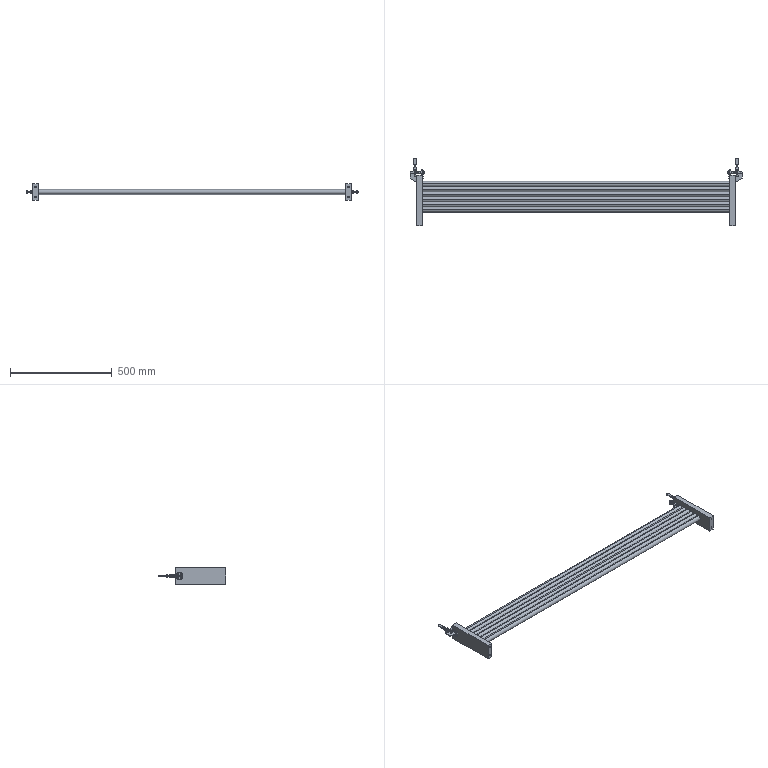Part | SolidWorks | features ReferencePattern 5, AEMSimFeature 1, LocalLPattern 1 | 18 solids | 576 faces | box 1633 x 333.3 x 80 mm | volume 5408151 mm3 | plane 290 | cylinder 196 | cone 74 | spline 16 | commonest cylinder face diameters 4.8 x48 6 x18 3.3 x16 10 x16 6.35 x12 19 x12